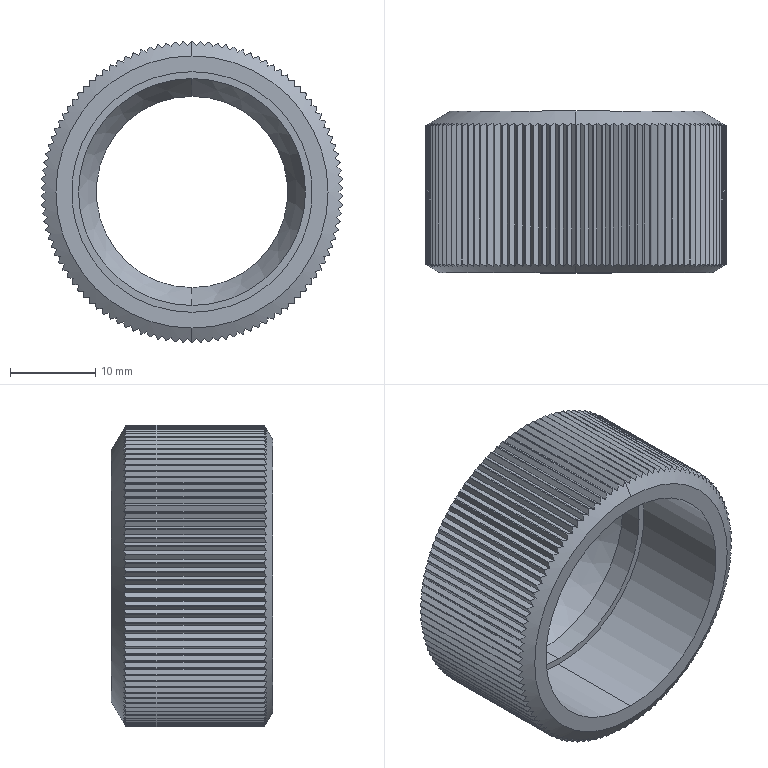Part | STEP file | 00649789_MUTTER_RAENDEL_MKRT-23-16.5 | 1 solid | 346 faces | box 35.488 x 19 x 35.5 mm | volume 6985 mm3 | plane 223 | cylinder 117 | cone 6 | commonest cylinder face diameters 35.5 x111 22.5 x2 26.7 x2 28.3 x2